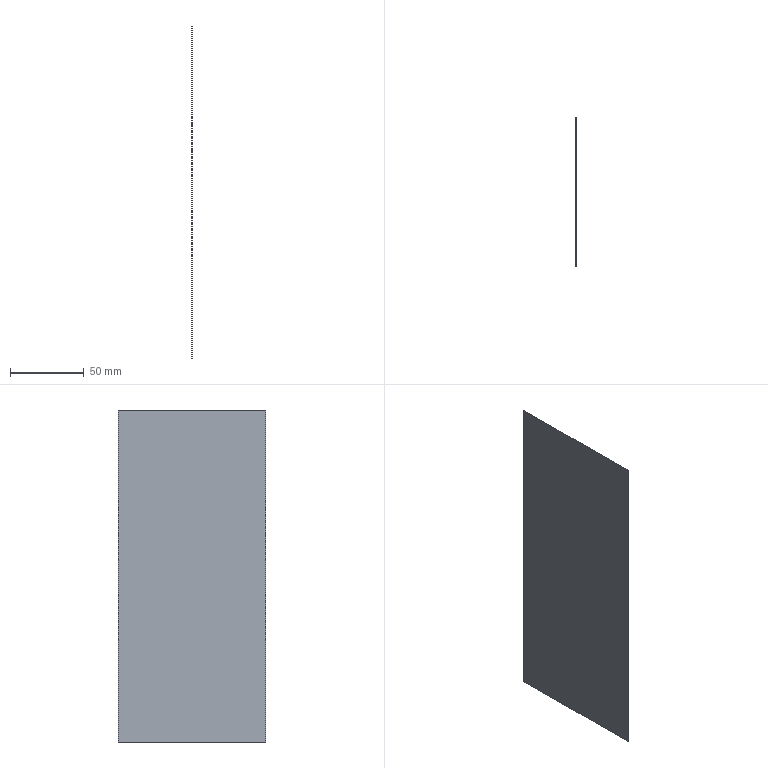Part | STEP file | A14-Product-2 | 1 solid | 6 faces | box 0.02 x 100 x 225 mm | volume 450 mm3 | plane 6
STEP:
#1=CARTESIAN_POINT('',(0.,0.,0.));
#2=DIRECTION('',(0.,0.,1.));
#3=DIRECTION('',(1.,0.,0.));
#4=AXIS2_PLACEMENT_3D('',#1,#2,#3);
#5=CARTESIAN_POINT('',(-0.01,-50.,-112.5));
#6=VERTEX_POINT('',#5);
#7=CARTESIAN_POINT('',(-0.01,50.,-112.5));
#8=VERTEX_POINT('',#7);
#9=CARTESIAN_POINT('',(-0.01,50.,-112.5));
#10=DIRECTION('',(0.,1.,0.));
#11=VECTOR('',#10,1.);
#12=LINE('',#9,#11);
#13=CARTESIAN_POINT('',(0.01,50.,-112.5));
#14=DIRECTION('',(0.,0.,1.));
#15=DIRECTION('',(1.,0.,0.));
#16=AXIS2_PLACEMENT_3D('',#13,#14,#15);
#17=PLANE('',#16);
#18=CARTESIAN_POINT('',(-0.02,0.));
#19=DIRECTION('',(0.,1.));
#20=VECTOR('',#19,1.);
#21=LINE('',#18,#20);
#22=(GEOMETRIC_REPRESENTATION_CONTEXT(2)PARAMETRIC_REPRESENTATION_CONTEXT()REPRESENTATION_CONTEXT('',''));
#23=DEFINITIONAL_REPRESENTATION('',(#21),#22);
#24=PCURVE('',#17,#23);
#25=CARTESIAN_POINT('',(-0.01,0.,0.));
#26=DIRECTION('',(1.,0.,0.));
#27=DIRECTION('',(0.,0.,-1.));
#28=AXIS2_PLACEMENT_3D('',#25,#26,#27);
#29=PLANE('',#28);
#30=CARTESIAN_POINT('',(112.5,50.));
#31=DIRECTION('',(0.,1.));
#32=VECTOR('',#31,1.);
#33=LINE('',#30,#32);
#34=(GEOMETRIC_REPRESENTATION_CONTEXT(2)PARAMETRIC_REPRESENTATION_CONTEXT()REPRESENTATION_CONTEXT('',''));
#35=DEFINITIONAL_REPRESENTATION('',(#33),#34);
#36=PCURVE('',#29,#35);
#37=SURFACE_CURVE('',#12,(#24,#36),.PCURVE_S1.);
#38=EDGE_CURVE('',#6,#8,#37,.T.);
#39=ORIENTED_EDGE('',*,*,#38,.T.);
#40=CARTESIAN_POINT('',(0.01,50.,-112.5));
#41=VERTEX_POINT('',#40);
#42=CARTESIAN_POINT('',(0.01,50.,-112.5));
#43=DIRECTION('',(-1.,0.,0.));
#44=VECTOR('',#43,1.);
#45=LINE('',#42,#44);
#46=CARTESIAN_POINT('',(0.,0.));
#47=DIRECTION('',(-1.,0.));
#48=VECTOR('',#47,1.);
#49=LINE('',#46,#48);
#50=(GEOMETRIC_REPRESENTATION_CONTEXT(2)PARAMETRIC_REPRESENTATION_CONTEXT()REPRESENTATION_CONTEXT('',''));
#51=DEFINITIONAL_REPRESENTATION('',(#49),#50);
#52=PCURVE('',#17,#51);
#53=CARTESIAN_POINT('',(0.01,50.,112.5));
#54=DIRECTION('',(0.,-1.,0.));
#55=DIRECTION('',(0.,0.,-1.));
#56=AXIS2_PLACEMENT_3D('',#53,#54,#55);
#57=PLANE('',#56);
#58=CARTESIAN_POINT('',(225.,0.));
#59=DIRECTION('',(0.,-1.));
#60=VECTOR('',#59,1.);
#61=LINE('',#58,#60);
#62=(GEOMETRIC_REPRESENTATION_CONTEXT(2)PARAMETRIC_REPRESENTATION_CONTEXT()REPRESENTATION_CONTEXT('',''));
#63=DEFINITIONAL_REPRESENTATION('',(#61),#62);
#64=PCURVE('',#57,#63);
#65=SURFACE_CURVE('',#45,(#52,#64),.PCURVE_S1.);
#66=EDGE_CURVE('',#41,#8,#65,.T.);
#67=ORIENTED_EDGE('',*,*,#66,.F.);
#68=CARTESIAN_POINT('',(0.01,-50.,-112.5));
#69=VERTEX_POINT('',#68);
#70=CARTESIAN_POINT('',(0.01,50.,-112.5));
#71=DIRECTION('',(0.,1.,0.));
#72=VECTOR('',#71,1.);
#73=LINE('',#70,#72);
#74=CARTESIAN_POINT('',(0.,0.));
#75=DIRECTION('',(0.,1.));
#76=VECTOR('',#75,1.);
#77=LINE('',#74,#76);
#78=(GEOMETRIC_REPRESENTATION_CONTEXT(2)PARAMETRIC_REPRESENTATION_CONTEXT()REPRESENTATION_CONTEXT('',''));
#79=DEFINITIONAL_REPRESENTATION('',(#77),#78);
#80=PCURVE('',#17,#79);
#81=CARTESIAN_POINT('',(0.01,0.,0.));
#82=DIRECTION('',(1.,0.,0.));
#83=DIRECTION('',(0.,0.,-1.));
#84=AXIS2_PLACEMENT_3D('',#81,#82,#83);
#85=PLANE('',#84);
#86=CARTESIAN_POINT('',(112.5,50.));
#87=DIRECTION('',(0.,1.));
#88=VECTOR('',#87,1.);
#89=LINE('',#86,#88);
#90=(GEOMETRIC_REPRESENTATION_CONTEXT(2)PARAMETRIC_REPRESENTATION_CONTEXT()REPRESENTATION_CONTEXT('',''));
#91=DEFINITIONAL_REPRESENTATION('',(#89),#90);
#92=PCURVE('',#85,#91);
#93=SURFACE_CURVE('',#73,(#80,#92),.PCURVE_S1.);
#94=EDGE_CURVE('',#69,#41,#93,.T.);
#95=ORIENTED_EDGE('',*,*,#94,.F.);
#96=CARTESIAN_POINT('',(0.01,-50.,-112.5));
#97=DIRECTION('',(-1.,0.,0.));
#98=VECTOR('',#97,1.);
#99=LINE('',#96,#98);
#100=CARTESIAN_POINT('',(0.,-100.));
#101=DIRECTION('',(-1.,0.));
#102=VECTOR('',#101,1.);
#103=LINE('',#100,#102);
#104=(GEOMETRIC_REPRESENTATION_CONTEXT(2)PARAMETRIC_REPRESENTATION_CONTEXT()REPRESENTATION_CONTEXT('',''));
#105=DEFINITIONAL_REPRESENTATION('',(#103),#104);
#106=PCURVE('',#17,#105);
#107=CARTESIAN_POINT('',(0.01,-50.,112.5));
#108=DIRECTION('',(0.,1.,0.));
#109=DIRECTION('',(0.,0.,1.));
#110=AXIS2_PLACEMENT_3D('',#107,#108,#109);
#111=PLANE('',#110);
#112=CARTESIAN_POINT('',(-225.,0.));
#113=DIRECTION('',(0.,-1.));
#114=VECTOR('',#113,1.);
#115=LINE('',#112,#114);
#116=(GEOMETRIC_REPRESENTATION_CONTEXT(2)PARAMETRIC_REPRESENTATION_CONTEXT()REPRESENTATION_CONTEXT('',''));
#117=DEFINITIONAL_REPRESENTATION('',(#115),#116);
#118=PCURVE('',#111,#117);
#119=SURFACE_CURVE('',#99,(#106,#118),.PCURVE_S1.);
#120=EDGE_CURVE('',#69,#6,#119,.T.);
#121=ORIENTED_EDGE('',*,*,#120,.T.);
#122=EDGE_LOOP('',(#39,#67,#95,#121));
#123=FACE_BOUND('',#122,.T.);
#124=ADVANCED_FACE('',(#123),#17,.F.);
#125=CARTESIAN_POINT('',(-0.01,50.,112.5));
#126=VERTEX_POINT('',#125);
#127=CARTESIAN_POINT('',(-0.01,50.,112.5));
#128=DIRECTION('',(0.,0.,1.));
#129=VECTOR('',#128,1.);
#130=LINE('',#127,#129);
#131=CARTESIAN_POINT('',(0.,-0.02));
#132=DIRECTION('',(-1.,0.));
#133=VECTOR('',#132,1.);
#134=LINE('',#131,#133);
#135=(GEOMETRIC_REPRESENTATION_CONTEXT(2)PARAMETRIC_REPRESENTATION_CONTEXT()REPRESENTATION_CONTEXT('',''));
#136=DEFINITIONAL_REPRESENTATION('',(#134),#135);
#137=PCURVE('',#57,#136);
#138=CARTESIAN_POINT('',(-112.5,50.));
#139=DIRECTION('',(-1.,0.));
#140=VECTOR('',#139,1.);
#141=LINE('',#138,#140);
#142=(GEOMETRIC_REPRESENTATION_CONTEXT(2)PARAMETRIC_REPRESENTATION_CONTEXT()REPRESENTATION_CONTEXT('',''));
#143=DEFINITIONAL_REPRESENTATION('',(#141),#142);
#144=PCURVE('',#29,#143);
#145=SURFACE_CURVE('',#130,(#137,#144),.PCURVE_S1.);
#146=EDGE_CURVE('',#8,#126,#145,.T.);
#147=ORIENTED_EDGE('',*,*,#146,.T.);
#148=CARTESIAN_POINT('',(0.01,50.,112.5));
#149=VERTEX_POINT('',#148);
#150=CARTESIAN_POINT('',(0.01,50.,112.5));
#151=DIRECTION('',(-1.,0.,0.));
#152=VECTOR('',#151,1.);
#153=LINE('',#150,#152);
#154=CARTESIAN_POINT('',(0.,0.));
#155=DIRECTION('',(0.,-1.));
#156=VECTOR('',#155,1.);
#157=LINE('',#154,#156);
#158=(GEOMETRIC_REPRESENTATION_CONTEXT(2)PARAMETRIC_REPRESENTATION_CONTEXT()REPRESENTATION_CONTEXT('',''));
#159=DEFINITIONAL_REPRESENTATION('',(#157),#158);
#160=PCURVE('',#57,#159);
#161=CARTESIAN_POINT('',(0.01,50.,112.5));
#162=DIRECTION('',(0.,0.,-1.));
#163=DIRECTION('',(0.,1.,0.));
#164=AXIS2_PLACEMENT_3D('',#161,#162,#163);
#165=PLANE('',#164);
#166=CARTESIAN_POINT('',(0.,0.));
#167=DIRECTION('',(0.,-1.));
#168=VECTOR('',#167,1.);
#169=LINE('',#166,#168);
#170=(GEOMETRIC_REPRESENTATION_CONTEXT(2)PARAMETRIC_REPRESENTATION_CONTEXT()REPRESENTATION_CONTEXT('',''));
#171=DEFINITIONAL_REPRESENTATION('',(#169),#170);
#172=PCURVE('',#165,#171);
#173=SURFACE_CURVE('',#153,(#160,#172),.PCURVE_S1.);
#174=EDGE_CURVE('',#149,#126,#173,.T.);
#175=ORIENTED_EDGE('',*,*,#174,.F.);
#176=CARTESIAN_POINT('',(0.01,50.,112.5));
#177=DIRECTION('',(0.,0.,1.));
#178=VECTOR('',#177,1.);
#179=LINE('',#176,#178);
#180=CARTESIAN_POINT('',(0.,0.));
#181=DIRECTION('',(-1.,0.));
#182=VECTOR('',#181,1.);
#183=LINE('',#180,#182);
#184=(GEOMETRIC_REPRESENTATION_CONTEXT(2)PARAMETRIC_REPRESENTATION_CONTEXT()REPRESENTATION_CONTEXT('',''));
#185=DEFINITIONAL_REPRESENTATION('',(#183),#184);
#186=PCURVE('',#57,#185);
#187=CARTESIAN_POINT('',(-112.5,50.));
#188=DIRECTION('',(-1.,0.));
#189=VECTOR('',#188,1.);
#190=LINE('',#187,#189);
#191=(GEOMETRIC_REPRESENTATION_CONTEXT(2)PARAMETRIC_REPRESENTATION_CONTEXT()REPRESENTATION_CONTEXT('',''));
#192=DEFINITIONAL_REPRESENTATION('',(#190),#191);
#193=PCURVE('',#85,#192);
#194=SURFACE_CURVE('',#179,(#186,#193),.PCURVE_S1.);
#195=EDGE_CURVE('',#41,#149,#194,.T.);
#196=ORIENTED_EDGE('',*,*,#195,.F.);
#197=ORIENTED_EDGE('',*,*,#66,.T.);
#198=EDGE_LOOP('',(#147,#175,#196,#197));
#199=FACE_BOUND('',#198,.T.);
#200=ADVANCED_FACE('',(#199),#57,.F.);
#201=CARTESIAN_POINT('',(-0.01,-50.,112.5));
#202=VERTEX_POINT('',#201);
#203=CARTESIAN_POINT('',(-0.01,50.,112.5));
#204=DIRECTION('',(0.,-1.,0.));
#205=VECTOR('',#204,1.);
#206=LINE('',#203,#205);
#207=CARTESIAN_POINT('',(0.,-0.02));
#208=DIRECTION('',(-1.,0.));
#209=VECTOR('',#208,1.);
#210=LINE('',#207,#209);
#211=(GEOMETRIC_REPRESENTATION_CONTEXT(2)PARAMETRIC_REPRESENTATION_CONTEXT()REPRESENTATION_CONTEXT('',''));
#212=DEFINITIONAL_REPRESENTATION('',(#210),#211);
#213=PCURVE('',#165,#212);
#214=CARTESIAN_POINT('',(-112.5,50.));
#215=DIRECTION('',(0.,-1.));
#216=VECTOR('',#215,1.);
#217=LINE('',#214,#216);
#218=(GEOMETRIC_REPRESENTATION_CONTEXT(2)PARAMETRIC_REPRESENTATION_CONTEXT()REPRESENTATION_CONTEXT('',''));
#219=DEFINITIONAL_REPRESENTATION('',(#217),#218);
#220=PCURVE('',#29,#219);
#221=SURFACE_CURVE('',#206,(#213,#220),.PCURVE_S1.);
#222=EDGE_CURVE('',#126,#202,#221,.T.);
#223=ORIENTED_EDGE('',*,*,#222,.T.);
#224=CARTESIAN_POINT('',(0.01,-50.,112.5));
#225=VERTEX_POINT('',#224);
#226=CARTESIAN_POINT('',(0.01,-50.,112.5));
#227=DIRECTION('',(-1.,0.,0.));
#228=VECTOR('',#227,1.);
#229=LINE('',#226,#228);
#230=CARTESIAN_POINT('',(-100.,0.));
#231=DIRECTION('',(0.,-1.));
#232=VECTOR('',#231,1.);
#233=LINE('',#230,#232);
#234=(GEOMETRIC_REPRESENTATION_CONTEXT(2)PARAMETRIC_REPRESENTATION_CONTEXT()REPRESENTATION_CONTEXT('',''));
#235=DEFINITIONAL_REPRESENTATION('',(#233),#234);
#236=PCURVE('',#165,#235);
#237=CARTESIAN_POINT('',(0.,0.));
#238=DIRECTION('',(0.,-1.));
#239=VECTOR('',#238,1.);
#240=LINE('',#237,#239);
#241=(GEOMETRIC_REPRESENTATION_CONTEXT(2)PARAMETRIC_REPRESENTATION_CONTEXT()REPRESENTATION_CONTEXT('',''));
#242=DEFINITIONAL_REPRESENTATION('',(#240),#241);
#243=PCURVE('',#111,#242);
#244=SURFACE_CURVE('',#229,(#236,#243),.PCURVE_S1.);
#245=EDGE_CURVE('',#225,#202,#244,.T.);
#246=ORIENTED_EDGE('',*,*,#245,.F.);
#247=CARTESIAN_POINT('',(0.01,50.,112.5));
#248=DIRECTION('',(0.,-1.,0.));
#249=VECTOR('',#248,1.);
#250=LINE('',#247,#249);
#251=CARTESIAN_POINT('',(0.,0.));
#252=DIRECTION('',(-1.,0.));
#253=VECTOR('',#252,1.);
#254=LINE('',#251,#253);
#255=(GEOMETRIC_REPRESENTATION_CONTEXT(2)PARAMETRIC_REPRESENTATION_CONTEXT()REPRESENTATION_CONTEXT('',''));
#256=DEFINITIONAL_REPRESENTATION('',(#254),#255);
#257=PCURVE('',#165,#256);
#258=CARTESIAN_POINT('',(-112.5,50.));
#259=DIRECTION('',(0.,-1.));
#260=VECTOR('',#259,1.);
#261=LINE('',#258,#260);
#262=(GEOMETRIC_REPRESENTATION_CONTEXT(2)PARAMETRIC_REPRESENTATION_CONTEXT()REPRESENTATION_CONTEXT('',''));
#263=DEFINITIONAL_REPRESENTATION('',(#261),#262);
#264=PCURVE('',#85,#263);
#265=SURFACE_CURVE('',#250,(#257,#264),.PCURVE_S1.);
#266=EDGE_CURVE('',#149,#225,#265,.T.);
#267=ORIENTED_EDGE('',*,*,#266,.F.);
#268=ORIENTED_EDGE('',*,*,#174,.T.);
#269=EDGE_LOOP('',(#223,#246,#267,#268));
#270=FACE_BOUND('',#269,.T.);
#271=ADVANCED_FACE('',(#270),#165,.F.);
#272=CARTESIAN_POINT('',(-0.01,-50.,112.5));
#273=DIRECTION('',(0.,0.,-1.));
#274=VECTOR('',#273,1.);
#275=LINE('',#272,#274);
#276=CARTESIAN_POINT('',(0.,-0.02));
#277=DIRECTION('',(-1.,0.));
#278=VECTOR('',#277,1.);
#279=LINE('',#276,#278);
#280=(GEOMETRIC_REPRESENTATION_CONTEXT(2)PARAMETRIC_REPRESENTATION_CONTEXT()REPRESENTATION_CONTEXT('',''));
#281=DEFINITIONAL_REPRESENTATION('',(#279),#280);
#282=PCURVE('',#111,#281);
#283=CARTESIAN_POINT('',(-112.5,-50.));
#284=DIRECTION('',(1.,0.));
#285=VECTOR('',#284,1.);
#286=LINE('',#283,#285);
#287=(GEOMETRIC_REPRESENTATION_CONTEXT(2)PARAMETRIC_REPRESENTATION_CONTEXT()REPRESENTATION_CONTEXT('',''));
#288=DEFINITIONAL_REPRESENTATION('',(#286),#287);
#289=PCURVE('',#29,#288);
#290=SURFACE_CURVE('',#275,(#282,#289),.PCURVE_S1.);
#291=EDGE_CURVE('',#202,#6,#290,.T.);
#292=ORIENTED_EDGE('',*,*,#291,.T.);
#293=ORIENTED_EDGE('',*,*,#120,.F.);
#294=CARTESIAN_POINT('',(0.01,-50.,112.5));
#295=DIRECTION('',(0.,0.,-1.));
#296=VECTOR('',#295,1.);
#297=LINE('',#294,#296);
#298=CARTESIAN_POINT('',(0.,0.));
#299=DIRECTION('',(-1.,0.));
#300=VECTOR('',#299,1.);
#301=LINE('',#298,#300);
#302=(GEOMETRIC_REPRESENTATION_CONTEXT(2)PARAMETRIC_REPRESENTATION_CONTEXT()REPRESENTATION_CONTEXT('',''));
#303=DEFINITIONAL_REPRESENTATION('',(#301),#302);
#304=PCURVE('',#111,#303);
#305=CARTESIAN_POINT('',(-112.5,-50.));
#306=DIRECTION('',(1.,0.));
#307=VECTOR('',#306,1.);
#308=LINE('',#305,#307);
#309=(GEOMETRIC_REPRESENTATION_CONTEXT(2)PARAMETRIC_REPRESENTATION_CONTEXT()REPRESENTATION_CONTEXT('',''));
#310=DEFINITIONAL_REPRESENTATION('',(#308),#309);
#311=PCURVE('',#85,#310);
#312=SURFACE_CURVE('',#297,(#304,#311),.PCURVE_S1.);
#313=EDGE_CURVE('',#225,#69,#312,.T.);
#314=ORIENTED_EDGE('',*,*,#313,.F.);
#315=ORIENTED_EDGE('',*,*,#245,.T.);
#316=EDGE_LOOP('',(#292,#293,#314,#315));
#317=FACE_BOUND('',#316,.T.);
#318=ADVANCED_FACE('',(#317),#111,.F.);
#319=ORIENTED_EDGE('',*,*,#94,.T.);
#320=ORIENTED_EDGE('',*,*,#195,.T.);
#321=ORIENTED_EDGE('',*,*,#266,.T.);
#322=ORIENTED_EDGE('',*,*,#313,.T.);
#323=EDGE_LOOP('',(#319,#320,#321,#322));
#324=FACE_BOUND('',#323,.T.);
#325=ADVANCED_FACE('',(#324),#85,.T.);
#326=ORIENTED_EDGE('',*,*,#38,.F.);
#327=ORIENTED_EDGE('',*,*,#291,.F.);
#328=ORIENTED_EDGE('',*,*,#222,.F.);
#329=ORIENTED_EDGE('',*,*,#146,.F.);
#330=EDGE_LOOP('',(#326,#327,#328,#329));
#331=FACE_BOUND('',#330,.T.);
#332=ADVANCED_FACE('',(#331),#29,.F.);
#333=CLOSED_SHELL('',(#124,#200,#271,#318,#325,#332));
#334=MANIFOLD_SOLID_BREP('',#333);
#335=(LENGTH_UNIT()NAMED_UNIT(*)SI_UNIT(.MILLI.,.METRE.));
#336=UNCERTAINTY_MEASURE_WITH_UNIT(LENGTH_MEASURE(0.0000001),#335,'','');
#337=(NAMED_UNIT(*)PLANE_ANGLE_UNIT()SI_UNIT($,.RADIAN.));
#338=(NAMED_UNIT(*)SI_UNIT($,.STERADIAN.)SOLID_ANGLE_UNIT());
#339=(GEOMETRIC_REPRESENTATION_CONTEXT(3)GLOBAL_UNCERTAINTY_ASSIGNED_CONTEXT((#336))GLOBAL_UNIT_ASSIGNED_CONTEXT((#335,#337,#338))REPRESENTATION_CONTEXT('',''));
#340=ADVANCED_BREP_SHAPE_REPRESENTATION('',(#4,#334),#339);